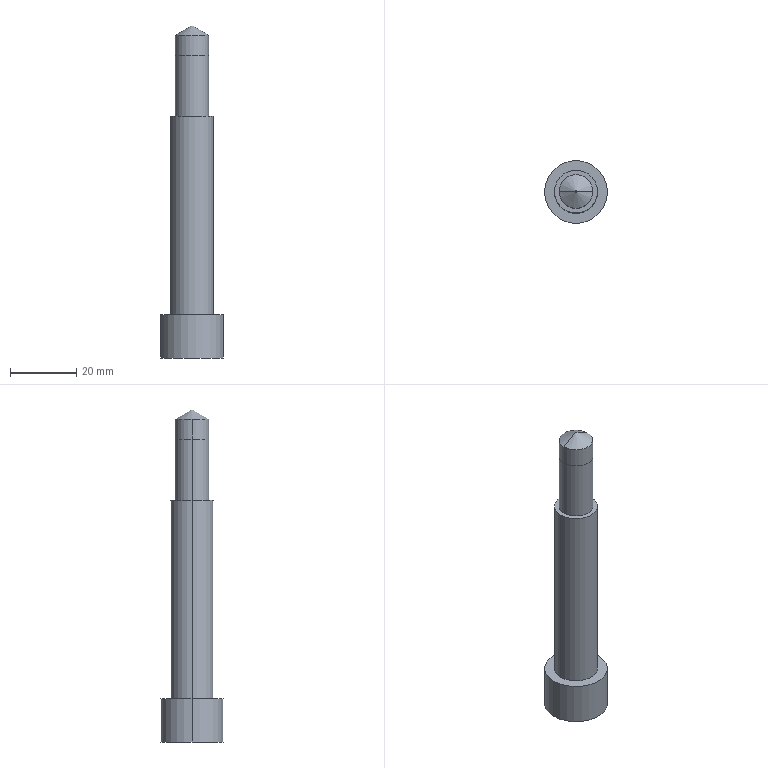Part | Creo | 1 solid | 14 faces | box 19 x 19 x 100.304 mm | volume 13732 mm3 | cylinder 8 | plane 4 | cone 2 | commonest cylinder face diameters 10.199 x2 10.2 x2 13 x2 19 x2
STEP:
#1=CARTESIAN_POINT('',(-70.1,250.,-29.));
#2=VERTEX_POINT('',#1);
#3=CARTESIAN_POINT('',(-59.9,250.,-29.));
#4=VERTEX_POINT('',#3);
#5=CARTESIAN_POINT('',(-65.,250.,-29.));
#6=DIRECTION('',(0.,0.,-1.));
#7=DIRECTION('',(-1.,0.,0.));
#8=AXIS2_PLACEMENT_3D('',#5,#6,#7);
#9=CIRCLE('',#8,5.1);
#10=EDGE_CURVE('',#2,#4,#9,.T.);
#11=ORIENTED_EDGE('',*,*,#10,.F.);
#12=CARTESIAN_POINT('',(-70.1,250.,-47.5));
#13=VERTEX_POINT('',#12);
#14=CARTESIAN_POINT('',(-70.1,250.,-29.));
#15=DIRECTION('',(-0.00001351,0.,-1.));
#16=VECTOR('',#15,18.5);
#17=LINE('',#14,#16);
#18=EDGE_CURVE('',#2,#13,#17,.T.);
#19=ORIENTED_EDGE('',*,*,#18,.T.);
#20=CARTESIAN_POINT('',(-59.9,250.,-47.5));
#21=VERTEX_POINT('',#20);
#22=CARTESIAN_POINT('',(-65.,250.,-47.5));
#23=DIRECTION('',(0.,0.,-1.));
#24=DIRECTION('',(-1.,0.,0.));
#25=AXIS2_PLACEMENT_3D('',#22,#23,#24);
#26=CIRCLE('',#25,5.1);
#27=EDGE_CURVE('',#13,#21,#26,.T.);
#28=ORIENTED_EDGE('',*,*,#27,.T.);
#29=CARTESIAN_POINT('',(-59.9,250.,-29.));
#30=DIRECTION('',(0.00001351,0.,-1.));
#31=VECTOR('',#30,18.5);
#32=LINE('',#29,#31);
#33=EDGE_CURVE('',#4,#21,#32,.T.);
#34=ORIENTED_EDGE('',*,*,#33,.F.);
#35=EDGE_LOOP('',(#11,#19,#28,#34));
#36=FACE_OUTER_BOUND('',#35,.F.);
#37=CARTESIAN_POINT('',(-65.,250.,-29.));
#38=DIRECTION('',(0.,0.,-1.));
#39=DIRECTION('',(-1.,0.,0.));
#40=AXIS2_PLACEMENT_3D('',#37,#38,#39);
#41=CYLINDRICAL_SURFACE('',#40,5.1);
#42=ADVANCED_FACE('',(#36),#41,.T.);
#43=CARTESIAN_POINT('',(-59.901,250.,-23.));
#44=VERTEX_POINT('',#43);
#45=CARTESIAN_POINT('',(-70.1,250.,-23.));
#46=VERTEX_POINT('',#45);
#47=CARTESIAN_POINT('',(-65.,250.,-23.));
#48=DIRECTION('',(0.,0.,1.));
#49=DIRECTION('',(1.,0.,0.));
#50=AXIS2_PLACEMENT_3D('',#47,#48,#49);
#51=CIRCLE('',#50,5.099);
#52=EDGE_CURVE('',#44,#46,#51,.T.);
#53=ORIENTED_EDGE('',*,*,#52,.T.);
#54=CARTESIAN_POINT('',(-70.1,250.,-29.));
#55=DIRECTION('',(0.00004167,0.,1.));
#56=VECTOR('',#55,6.);
#57=LINE('',#54,#56);
#58=EDGE_CURVE('',#2,#46,#57,.T.);
#59=ORIENTED_EDGE('',*,*,#58,.F.);
#60=ORIENTED_EDGE('',*,*,#10,.T.);
#61=CARTESIAN_POINT('',(-59.9,250.,-29.));
#62=DIRECTION('',(-0.00004167,0.,1.));
#63=VECTOR('',#62,6.);
#64=LINE('',#61,#63);
#65=EDGE_CURVE('',#4,#44,#64,.T.);
#66=ORIENTED_EDGE('',*,*,#65,.T.);
#67=EDGE_LOOP('',(#53,#59,#60,#66));
#68=FACE_OUTER_BOUND('',#67,.F.);
#69=CARTESIAN_POINT('',(-65.,250.,-29.));
#70=DIRECTION('',(0.,0.,1.));
#71=DIRECTION('',(1.,0.,0.));
#72=AXIS2_PLACEMENT_3D('',#69,#70,#71);
#73=CYLINDRICAL_SURFACE('',#72,5.099);
#74=ADVANCED_FACE('',(#68),#73,.T.);
#75=CARTESIAN_POINT('',(-64.757,250.,-20.196));
#76=VERTEX_POINT('',#75);
#77=CARTESIAN_POINT('',(-65.243,250.,-20.196));
#78=VERTEX_POINT('',#77);
#79=CARTESIAN_POINT('',(-65.,250.,-20.196));
#80=DIRECTION('',(0.,0.,1.));
#81=DIRECTION('',(1.,0.,0.));
#82=AXIS2_PLACEMENT_3D('',#79,#80,#81);
#83=CIRCLE('',#82,0.2432);
#84=EDGE_CURVE('',#76,#78,#83,.T.);
#85=ORIENTED_EDGE('',*,*,#84,.T.);
#86=CARTESIAN_POINT('',(-65.243,250.,-20.196));
#87=DIRECTION('',(-0.866,0.,-0.5));
#88=VECTOR('',#87,5.608);
#89=LINE('',#86,#88);
#90=EDGE_CURVE('',#78,#46,#89,.T.);
#91=ORIENTED_EDGE('',*,*,#90,.T.);
#92=ORIENTED_EDGE('',*,*,#52,.F.);
#93=CARTESIAN_POINT('',(-64.757,250.,-20.196));
#94=DIRECTION('',(0.866,0.,-0.5));
#95=VECTOR('',#94,5.608);
#96=LINE('',#93,#95);
#97=EDGE_CURVE('',#76,#44,#96,.T.);
#98=ORIENTED_EDGE('',*,*,#97,.F.);
#99=EDGE_LOOP('',(#85,#91,#92,#98));
#100=FACE_OUTER_BOUND('',#99,.F.);
#101=CARTESIAN_POINT('',(-65.,250.,-21.598));
#102=DIRECTION('',(0.,0.,-1.));
#103=DIRECTION('',(-1.,0.,0.));
#104=AXIS2_PLACEMENT_3D('',#101,#102,#103);
#105=CONICAL_SURFACE('',#104,2.671,60.);
#106=ADVANCED_FACE('',(#100),#105,.T.);
#107=ORIENTED_EDGE('',*,*,#84,.F.);
#108=CARTESIAN_POINT('',(-65.,250.,-20.196));
#109=DIRECTION('',(0.,0.,1.));
#110=DIRECTION('',(-1.,0.,0.));
#111=AXIS2_PLACEMENT_3D('',#108,#109,#110);
#112=CIRCLE('',#111,0.2432);
#113=EDGE_CURVE('',#78,#76,#112,.T.);
#114=ORIENTED_EDGE('',*,*,#113,.F.);
#115=EDGE_LOOP('',(#107,#114));
#116=FACE_OUTER_BOUND('',#115,.F.);
#117=CARTESIAN_POINT('',(-65.,250.,-20.196));
#118=DIRECTION('',(0.,0.,1.));
#119=DIRECTION('',(1.,0.,0.));
#120=AXIS2_PLACEMENT_3D('',#117,#118,#119);
#121=PLANE('',#120);
#122=ADVANCED_FACE('',(#116),#121,.T.);
#123=ORIENTED_EDGE('',*,*,#113,.T.);
#124=ORIENTED_EDGE('',*,*,#97,.T.);
#125=CARTESIAN_POINT('',(-65.,250.,-23.));
#126=DIRECTION('',(0.,0.,1.));
#127=DIRECTION('',(-1.,0.,0.));
#128=AXIS2_PLACEMENT_3D('',#125,#126,#127);
#129=CIRCLE('',#128,5.099);
#130=EDGE_CURVE('',#46,#44,#129,.T.);
#131=ORIENTED_EDGE('',*,*,#130,.F.);
#132=ORIENTED_EDGE('',*,*,#90,.F.);
#133=EDGE_LOOP('',(#123,#124,#131,#132));
#134=FACE_OUTER_BOUND('',#133,.F.);
#135=CARTESIAN_POINT('',(-65.,250.,-21.598));
#136=DIRECTION('',(0.,0.,-1.));
#137=DIRECTION('',(-1.,0.,0.));
#138=AXIS2_PLACEMENT_3D('',#135,#136,#137);
#139=CONICAL_SURFACE('',#138,2.671,60.);
#140=ADVANCED_FACE('',(#134),#139,.T.);
#141=ORIENTED_EDGE('',*,*,#130,.T.);
#142=ORIENTED_EDGE('',*,*,#65,.F.);
#143=CARTESIAN_POINT('',(-65.,250.,-29.));
#144=DIRECTION('',(0.,0.,-1.));
#145=DIRECTION('',(1.,0.,0.));
#146=AXIS2_PLACEMENT_3D('',#143,#144,#145);
#147=CIRCLE('',#146,5.1);
#148=EDGE_CURVE('',#4,#2,#147,.T.);
#149=ORIENTED_EDGE('',*,*,#148,.T.);
#150=ORIENTED_EDGE('',*,*,#58,.T.);
#151=EDGE_LOOP('',(#141,#142,#149,#150));
#152=FACE_OUTER_BOUND('',#151,.F.);
#153=CARTESIAN_POINT('',(-65.,250.,-29.));
#154=DIRECTION('',(0.,0.,1.));
#155=DIRECTION('',(1.,0.,0.));
#156=AXIS2_PLACEMENT_3D('',#153,#154,#155);
#157=CYLINDRICAL_SURFACE('',#156,5.099);
#158=ADVANCED_FACE('',(#152),#157,.T.);
#159=ORIENTED_EDGE('',*,*,#148,.F.);
#160=ORIENTED_EDGE('',*,*,#33,.T.);
#161=CARTESIAN_POINT('',(-65.,250.,-47.5));
#162=DIRECTION('',(0.,0.,-1.));
#163=DIRECTION('',(1.,0.,0.));
#164=AXIS2_PLACEMENT_3D('',#161,#162,#163);
#165=CIRCLE('',#164,5.1);
#166=EDGE_CURVE('',#21,#13,#165,.T.);
#167=ORIENTED_EDGE('',*,*,#166,.T.);
#168=ORIENTED_EDGE('',*,*,#18,.F.);
#169=EDGE_LOOP('',(#159,#160,#167,#168));
#170=FACE_OUTER_BOUND('',#169,.F.);
#171=CARTESIAN_POINT('',(-65.,250.,-29.));
#172=DIRECTION('',(0.,0.,-1.));
#173=DIRECTION('',(-1.,0.,0.));
#174=AXIS2_PLACEMENT_3D('',#171,#172,#173);
#175=CYLINDRICAL_SURFACE('',#174,5.1);
#176=ADVANCED_FACE('',(#170),#175,.T.);
#177=CARTESIAN_POINT('',(-71.5,250.,-47.5));
#178=VERTEX_POINT('',#177);
#179=CARTESIAN_POINT('',(-58.5,250.,-47.5));
#180=VERTEX_POINT('',#179);
#181=CARTESIAN_POINT('',(-65.,250.,-47.5));
#182=DIRECTION('',(0.,0.,1.));
#183=DIRECTION('',(-1.,0.,0.));
#184=AXIS2_PLACEMENT_3D('',#181,#182,#183);
#185=CIRCLE('',#184,6.5);
#186=EDGE_CURVE('',#178,#180,#185,.T.);
#187=ORIENTED_EDGE('',*,*,#186,.F.);
#188=CARTESIAN_POINT('',(-65.,250.,-47.5));
#189=DIRECTION('',(0.,0.,1.));
#190=DIRECTION('',(1.,0.,0.));
#191=AXIS2_PLACEMENT_3D('',#188,#189,#190);
#192=CIRCLE('',#191,6.5);
#193=EDGE_CURVE('',#180,#178,#192,.T.);
#194=ORIENTED_EDGE('',*,*,#193,.F.);
#195=EDGE_LOOP('',(#187,#194));
#196=FACE_OUTER_BOUND('',#195,.F.);
#197=ORIENTED_EDGE('',*,*,#166,.F.);
#198=ORIENTED_EDGE('',*,*,#27,.F.);
#199=EDGE_LOOP('',(#197,#198));
#200=FACE_BOUND('',#199,.F.);
#201=CARTESIAN_POINT('',(-65.,250.,-47.5));
#202=DIRECTION('',(0.,0.,1.));
#203=DIRECTION('',(1.,0.,0.));
#204=AXIS2_PLACEMENT_3D('',#201,#202,#203);
#205=PLANE('',#204);
#206=ADVANCED_FACE('',(#196,#200),#205,.T.);
#207=CARTESIAN_POINT('',(-58.5,250.,-107.5));
#208=VERTEX_POINT('',#207);
#209=CARTESIAN_POINT('',(-71.5,250.,-107.5));
#210=VERTEX_POINT('',#209);
#211=CARTESIAN_POINT('',(-65.,250.,-107.5));
#212=DIRECTION('',(0.,0.,-1.));
#213=DIRECTION('',(1.,0.,0.));
#214=AXIS2_PLACEMENT_3D('',#211,#212,#213);
#215=CIRCLE('',#214,6.5);
#216=EDGE_CURVE('',#208,#210,#215,.T.);
#217=ORIENTED_EDGE('',*,*,#216,.T.);
#218=CARTESIAN_POINT('',(-71.5,250.,-47.5));
#219=DIRECTION('',(0.,0.,-1.));
#220=VECTOR('',#219,60.);
#221=LINE('',#218,#220);
#222=EDGE_CURVE('',#178,#210,#221,.T.);
#223=ORIENTED_EDGE('',*,*,#222,.F.);
#224=ORIENTED_EDGE('',*,*,#186,.T.);
#225=CARTESIAN_POINT('',(-58.5,250.,-47.5));
#226=DIRECTION('',(0.,0.,-1.));
#227=VECTOR('',#226,60.);
#228=LINE('',#225,#227);
#229=EDGE_CURVE('',#180,#208,#228,.T.);
#230=ORIENTED_EDGE('',*,*,#229,.T.);
#231=EDGE_LOOP('',(#217,#223,#224,#230));
#232=FACE_OUTER_BOUND('',#231,.F.);
#233=CARTESIAN_POINT('',(-65.,250.,-50.));
#234=DIRECTION('',(0.,0.,-1.));
#235=DIRECTION('',(-1.,0.,0.));
#236=AXIS2_PLACEMENT_3D('',#233,#234,#235);
#237=CYLINDRICAL_SURFACE('',#236,6.5);
#238=ADVANCED_FACE('',(#232),#237,.T.);
#239=CARTESIAN_POINT('',(-74.5,250.,-107.5));
#240=VERTEX_POINT('',#239);
#241=CARTESIAN_POINT('',(-55.5,250.,-107.5));
#242=VERTEX_POINT('',#241);
#243=CARTESIAN_POINT('',(-65.,250.,-107.5));
#244=DIRECTION('',(0.,0.,1.));
#245=DIRECTION('',(-1.,0.,0.));
#246=AXIS2_PLACEMENT_3D('',#243,#244,#245);
#247=CIRCLE('',#246,9.5);
#248=EDGE_CURVE('',#240,#242,#247,.T.);
#249=ORIENTED_EDGE('',*,*,#248,.F.);
#250=CARTESIAN_POINT('',(-65.,250.,-107.5));
#251=DIRECTION('',(0.,0.,1.));
#252=DIRECTION('',(1.,0.,0.));
#253=AXIS2_PLACEMENT_3D('',#250,#251,#252);
#254=CIRCLE('',#253,9.5);
#255=EDGE_CURVE('',#242,#240,#254,.T.);
#256=ORIENTED_EDGE('',*,*,#255,.F.);
#257=EDGE_LOOP('',(#249,#256));
#258=FACE_OUTER_BOUND('',#257,.F.);
#259=CARTESIAN_POINT('',(-65.,250.,-107.5));
#260=DIRECTION('',(0.,0.,-1.));
#261=DIRECTION('',(-1.,0.,0.));
#262=AXIS2_PLACEMENT_3D('',#259,#260,#261);
#263=CIRCLE('',#262,6.5);
#264=EDGE_CURVE('',#210,#208,#263,.T.);
#265=ORIENTED_EDGE('',*,*,#264,.F.);
#266=ORIENTED_EDGE('',*,*,#216,.F.);
#267=EDGE_LOOP('',(#265,#266));
#268=FACE_BOUND('',#267,.F.);
#269=CARTESIAN_POINT('',(-65.,250.,-107.5));
#270=DIRECTION('',(0.,0.,1.));
#271=DIRECTION('',(1.,0.,0.));
#272=AXIS2_PLACEMENT_3D('',#269,#270,#271);
#273=PLANE('',#272);
#274=ADVANCED_FACE('',(#258,#268),#273,.T.);
#275=ORIENTED_EDGE('',*,*,#264,.T.);
#276=ORIENTED_EDGE('',*,*,#229,.F.);
#277=ORIENTED_EDGE('',*,*,#193,.T.);
#278=ORIENTED_EDGE('',*,*,#222,.T.);
#279=EDGE_LOOP('',(#275,#276,#277,#278));
#280=FACE_OUTER_BOUND('',#279,.F.);
#281=CARTESIAN_POINT('',(-65.,250.,-50.));
#282=DIRECTION('',(0.,0.,-1.));
#283=DIRECTION('',(-1.,0.,0.));
#284=AXIS2_PLACEMENT_3D('',#281,#282,#283);
#285=CYLINDRICAL_SURFACE('',#284,6.5);
#286=ADVANCED_FACE('',(#280),#285,.T.);
#287=CARTESIAN_POINT('',(-55.5,250.,-120.5));
#288=VERTEX_POINT('',#287);
#289=CARTESIAN_POINT('',(-74.5,250.,-120.5));
#290=VERTEX_POINT('',#289);
#291=CARTESIAN_POINT('',(-65.,250.,-120.5));
#292=DIRECTION('',(0.,0.,-1.));
#293=DIRECTION('',(1.,0.,0.));
#294=AXIS2_PLACEMENT_3D('',#291,#292,#293);
#295=CIRCLE('',#294,9.5);
#296=EDGE_CURVE('',#288,#290,#295,.T.);
#297=ORIENTED_EDGE('',*,*,#296,.T.);
#298=CARTESIAN_POINT('',(-74.5,250.,-107.5));
#299=DIRECTION('',(0.,0.,-1.));
#300=VECTOR('',#299,13.);
#301=LINE('',#298,#300);
#302=EDGE_CURVE('',#240,#290,#301,.T.);
#303=ORIENTED_EDGE('',*,*,#302,.F.);
#304=ORIENTED_EDGE('',*,*,#248,.T.);
#305=CARTESIAN_POINT('',(-55.5,250.,-107.5));
#306=DIRECTION('',(0.,0.,-1.));
#307=VECTOR('',#306,13.);
#308=LINE('',#305,#307);
#309=EDGE_CURVE('',#242,#288,#308,.T.);
#310=ORIENTED_EDGE('',*,*,#309,.T.);
#311=EDGE_LOOP('',(#297,#303,#304,#310));
#312=FACE_OUTER_BOUND('',#311,.F.);
#313=CARTESIAN_POINT('',(-65.,250.,-107.5));
#314=DIRECTION('',(0.,0.,-1.));
#315=DIRECTION('',(-1.,0.,0.));
#316=AXIS2_PLACEMENT_3D('',#313,#314,#315);
#317=CYLINDRICAL_SURFACE('',#316,9.5);
#318=ADVANCED_FACE('',(#312),#317,.T.);
#319=CARTESIAN_POINT('',(-65.,250.,-120.5));
#320=DIRECTION('',(0.,0.,-1.));
#321=DIRECTION('',(-1.,0.,0.));
#322=AXIS2_PLACEMENT_3D('',#319,#320,#321);
#323=CIRCLE('',#322,9.5);
#324=EDGE_CURVE('',#290,#288,#323,.T.);
#325=ORIENTED_EDGE('',*,*,#324,.F.);
#326=ORIENTED_EDGE('',*,*,#296,.F.);
#327=EDGE_LOOP('',(#325,#326));
#328=FACE_OUTER_BOUND('',#327,.F.);
#329=CARTESIAN_POINT('',(-65.,250.,-120.5));
#330=DIRECTION('',(0.,0.,-1.));
#331=DIRECTION('',(-1.,0.,0.));
#332=AXIS2_PLACEMENT_3D('',#329,#330,#331);
#333=PLANE('',#332);
#334=ADVANCED_FACE('',(#328),#333,.T.);
#335=ORIENTED_EDGE('',*,*,#324,.T.);
#336=ORIENTED_EDGE('',*,*,#309,.F.);
#337=ORIENTED_EDGE('',*,*,#255,.T.);
#338=ORIENTED_EDGE('',*,*,#302,.T.);
#339=EDGE_LOOP('',(#335,#336,#337,#338));
#340=FACE_OUTER_BOUND('',#339,.F.);
#341=CARTESIAN_POINT('',(-65.,250.,-107.5));
#342=DIRECTION('',(0.,0.,-1.));
#343=DIRECTION('',(-1.,0.,0.));
#344=AXIS2_PLACEMENT_3D('',#341,#342,#343);
#345=CYLINDRICAL_SURFACE('',#344,9.5);
#346=ADVANCED_FACE('',(#340),#345,.T.);
#347=CLOSED_SHELL('',(#42,#74,#106,#122,#140,#158,#176,#206,#238,#274,#286,#318,#334,#346));
#348=MANIFOLD_SOLID_BREP('',#347);
#349=(LENGTH_UNIT()NAMED_UNIT(*)SI_UNIT(.MILLI.,.METRE.));
#350=UNCERTAINTY_MEASURE_WITH_UNIT(LENGTH_MEASURE(0.01038),#349,'','');
#351=(NAMED_UNIT(*)PLANE_ANGLE_UNIT()SI_UNIT($,.RADIAN.));
#352=PLANE_ANGLE_MEASURE_WITH_UNIT(PLANE_ANGLE_MEASURE(0.01745),#351);
#353=(CONVERSION_BASED_UNIT('DEGREE',#352)NAMED_UNIT(*)PLANE_ANGLE_UNIT());
#354=(NAMED_UNIT(*)SI_UNIT($,.STERADIAN.)SOLID_ANGLE_UNIT());
#355=(GEOMETRIC_REPRESENTATION_CONTEXT(3)GLOBAL_UNCERTAINTY_ASSIGNED_CONTEXT((#350))GLOBAL_UNIT_ASSIGNED_CONTEXT((#349,#353,#354))REPRESENTATION_CONTEXT('',''));
#356=ADVANCED_BREP_SHAPE_REPRESENTATION('',(#348),#355);